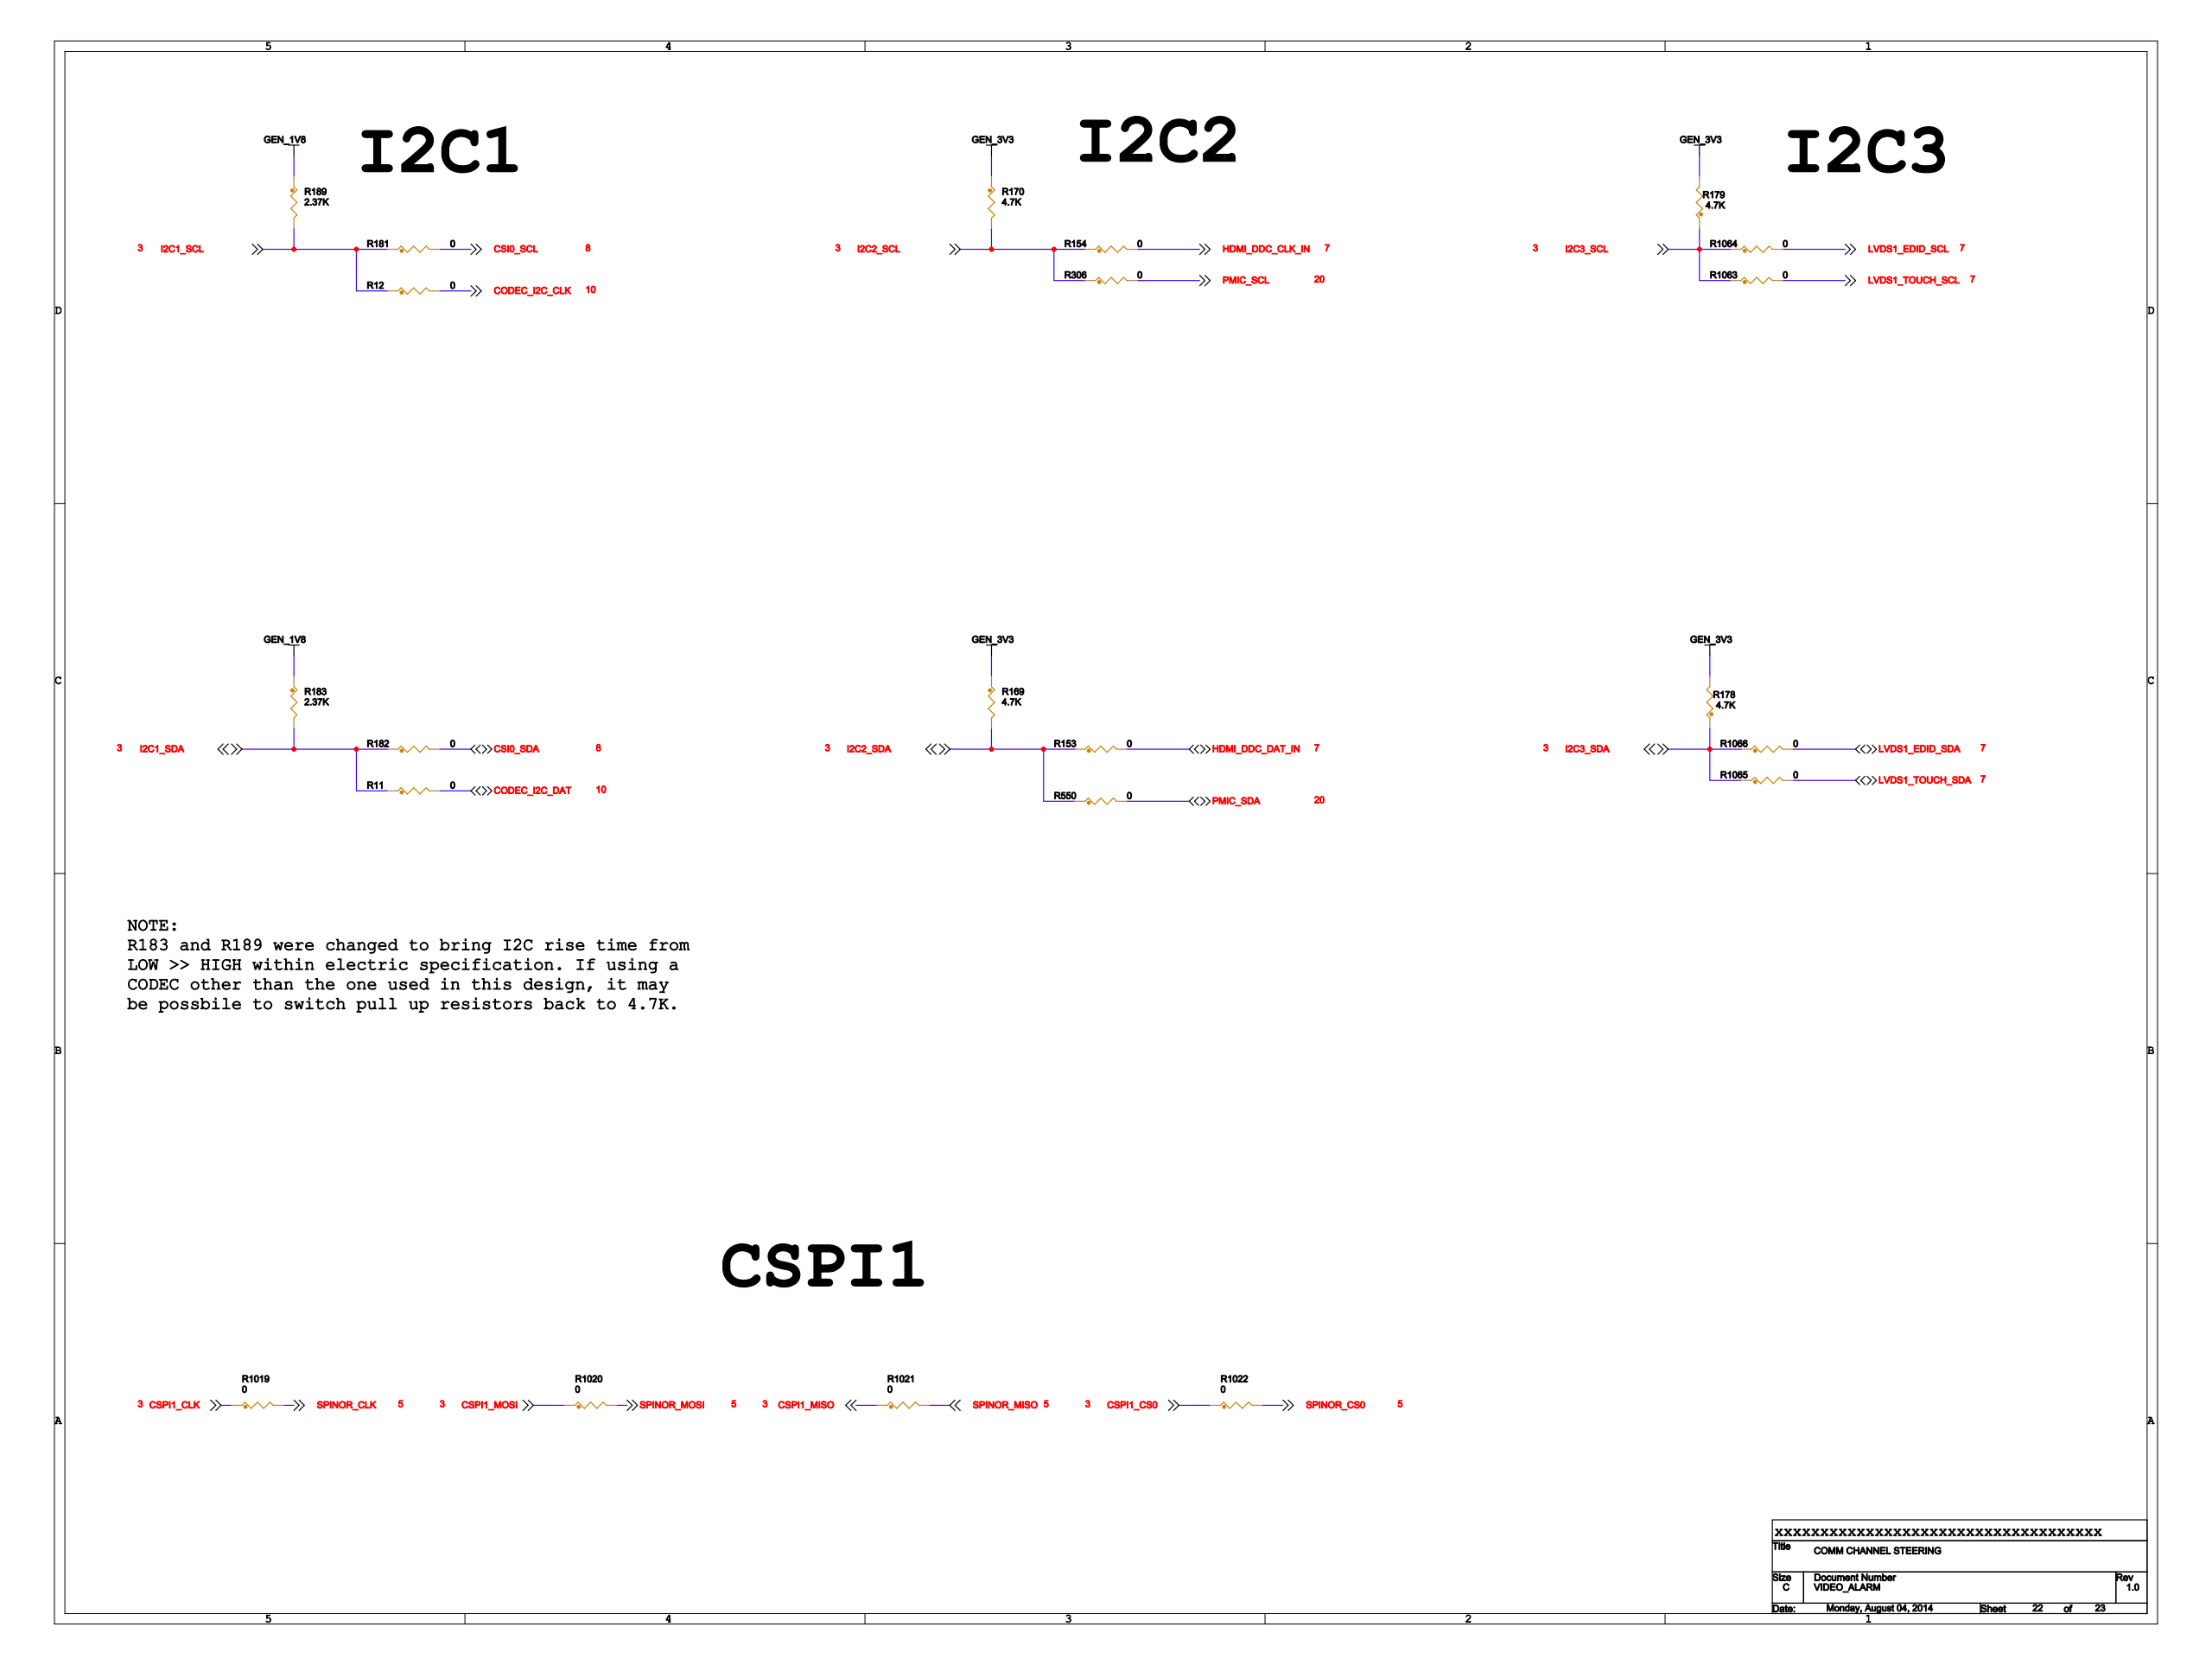Circuit board | Cadence Allegro | 994 parts | 728 nets | one sheet of the schematic
Parts on this sheet (reference | value | footprint):
R11 | 0 | 0603_CC
R12 | 0 | 0603_CC
R169 | 4.7K | 0603_CC
R170 | 4.7K | 0603_CC
R178 | 4.7K | 0603_CC
R179 | 4.7K | 0603_CC
R181 | 0 | 0603_CC
R182 | 0 | 0603_CC
R183 | 2.37K | 0603_CC
R189 | 2.37K | 0603_CC
R306 | 0 | 0603_CC
R550 | 0 | 0603_CC
R1019 | 0 | 0805_CC
R1020 | 0 | 0805_CC
R1021 | 0 | 0805_CC
R1022 | 0 | 0805_CC
R1063 | 0 | 0603_CC
R1064 | 0 | 0603_CC
R1065 | 0 | 0603_CC
R1066 | 0 | 0603_CC
Nets of these parts (net: part-pin ...):
PMIC_SCL: R306-2
PMIC_SDA: R550-2
GEN_3V3: R169-1 R170-1 R178-2 R179-2
GEN_1V8: R183-1 R189-1
CSI0_SDA: R182-2
CSI0_SCL: R181-2
I2C1_SDA: R11-1 R182-1 R183-2
I2C1_SCL: R12-1 R181-1 R189-2
I2C2_SCL: R170-2 R306-1
I2C2_SDA: R169-2 R550-1
LVDS1_EDID_SCL: R1064-2
LVDS1_EDID_SDA: R1066-2
LVDS1_TOUCH_SCL: R1063-2
LVDS1_TOUCH_SDA: R1065-2
CODEC_I2C_CLK: R12-2
CODEC_I2C_DAT: R11-2
I2C3_SDA: R178-1 R1065-1 R1066-1
I2C3_SCL: R179-1 R1063-1 R1064-1
SPINOR_CLK: R1019-2
SPINOR_MOSI: R1020-2
SPINOR_MISO: R1021-2
SPINOR_CS0: R1022-2
CSPI1_CS0: R1022-1
CSPI1_MISO: R1021-1
CSPI1_MOSI: R1020-1
CSPI1_CLK: R1019-1